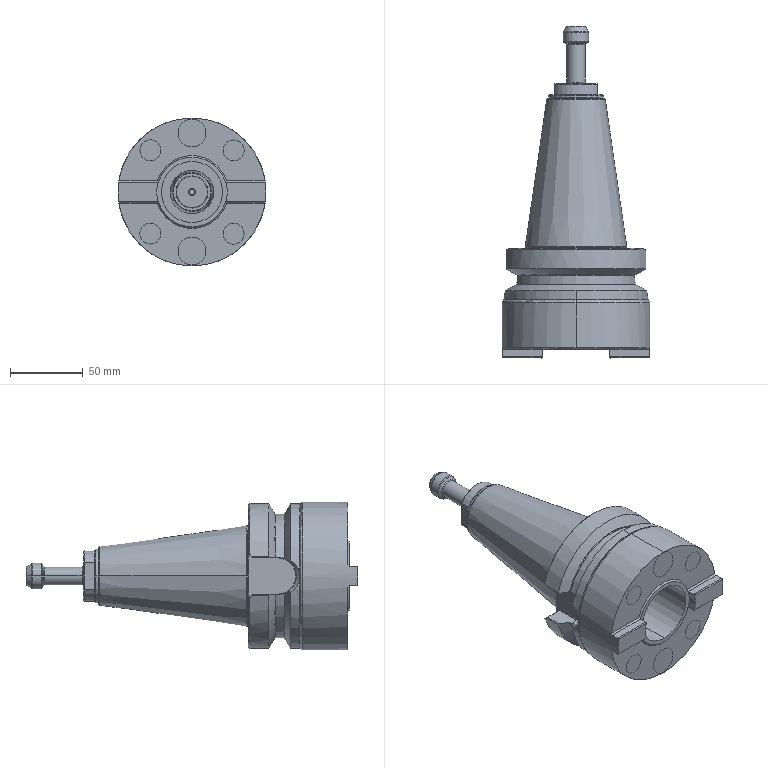Part | SolidWorks | features BaseBody 1 | 1 solid | 250 faces | box 102 x 228.798 x 102 mm | volume 662464 mm3 | plane 90 | cylinder 70 | cone 58 | torus 32 | commonest cylinder face diameters 0.75 x8 5.035 x8 99.975 x6 2.8 x4 6 x4 6.375 x4